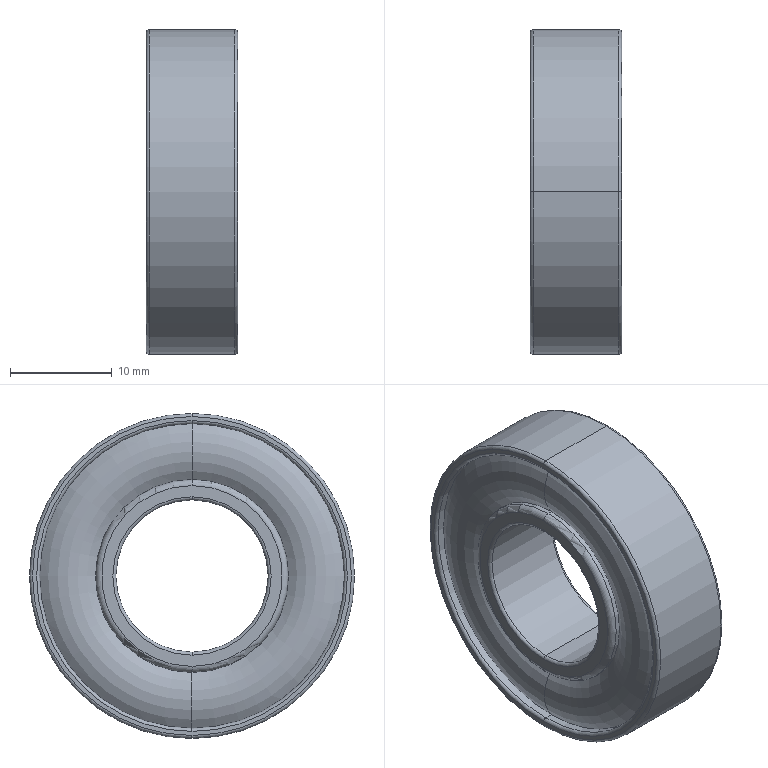Part | STEP file | 1 solid | 36 faces | box 9 x 32 x 32 mm | volume 5285 mm3 | torus 20 | cylinder 12 | plane 4 | commonest cylinder face diameters 19 x4 30 x4 15 x2 32 x2